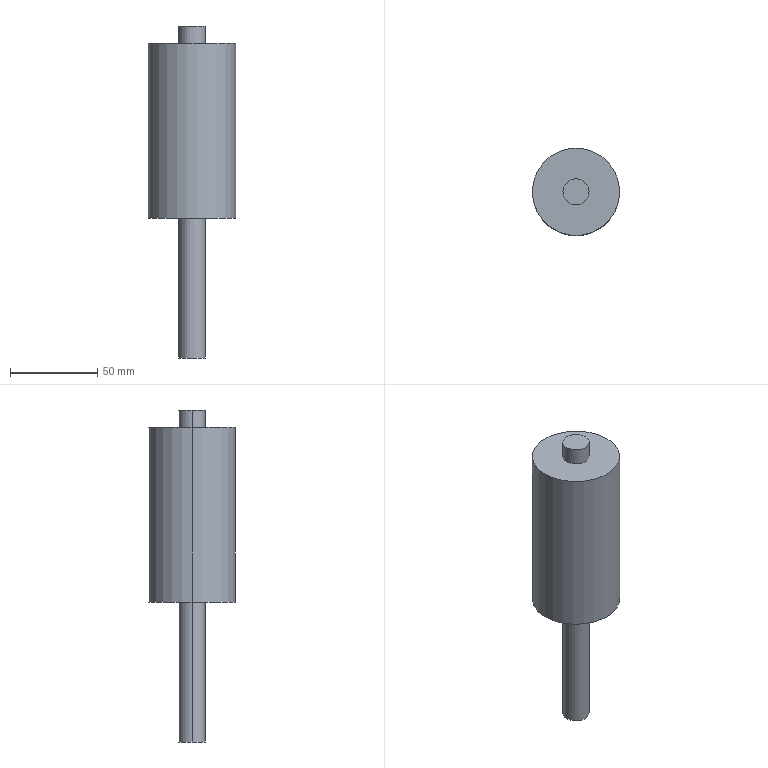Part | SolidWorks | features ICE 2, Extrusion 1 | 1 solid | 10 faces | box 50 x 50 x 190 mm | volume 212254 mm3 | cylinder 6 | plane 4 | commonest cylinder face diameters 15 x4 50 x2
STEP:
#1=CARTESIAN_POINT('',(-7.5,0.,-80.));
#2=VERTEX_POINT('',#1);
#3=CARTESIAN_POINT('',(7.5,0.,-80.));
#4=VERTEX_POINT('',#3);
#5=CARTESIAN_POINT('',(0.,0.,-80.));
#6=DIRECTION('',(0.,0.,-1.));
#7=DIRECTION('',(-1.,0.,0.));
#8=AXIS2_PLACEMENT_3D('',#5,#6,#7);
#9=CIRCLE('',#8,7.5);
#10=EDGE_CURVE('',#2,#4,#9,.T.);
#11=ORIENTED_EDGE('',*,*,#10,.F.);
#12=CARTESIAN_POINT('',(-7.5,0.,0.));
#13=VERTEX_POINT('',#12);
#14=CARTESIAN_POINT('',(-7.5,0.,-80.));
#15=DIRECTION('',(0.,0.,1.));
#16=VECTOR('',#15,1000.);
#17=LINE('',#14,#16);
#18=EDGE_CURVE('',#2,#13,#17,.T.);
#19=ORIENTED_EDGE('',*,*,#18,.T.);
#20=CARTESIAN_POINT('',(7.5,0.,0.));
#21=VERTEX_POINT('',#20);
#22=CARTESIAN_POINT('',(0.,0.,0.));
#23=DIRECTION('',(0.,0.,-1.));
#24=DIRECTION('',(-1.,0.,0.));
#25=AXIS2_PLACEMENT_3D('',#22,#23,#24);
#26=CIRCLE('',#25,7.5);
#27=EDGE_CURVE('',#13,#21,#26,.T.);
#28=ORIENTED_EDGE('',*,*,#27,.T.);
#29=CARTESIAN_POINT('',(7.5,0.,-80.));
#30=DIRECTION('',(0.,0.,1.));
#31=VECTOR('',#30,1000.);
#32=LINE('',#29,#31);
#33=EDGE_CURVE('',#4,#21,#32,.T.);
#34=ORIENTED_EDGE('',*,*,#33,.F.);
#35=EDGE_LOOP('',(#11,#19,#28,#34));
#36=FACE_OUTER_BOUND('',#35,.T.);
#37=CARTESIAN_POINT('',(0.,0.,-80.));
#38=DIRECTION('',(0.,0.,1.));
#39=DIRECTION('',(1.,0.,0.));
#40=AXIS2_PLACEMENT_3D('',#37,#38,#39);
#41=CYLINDRICAL_SURFACE('',#40,7.5);
#42=ADVANCED_FACE('',(#36),#41,.T.);
#43=CARTESIAN_POINT('',(7.5,0.,110.));
#44=VERTEX_POINT('',#43);
#45=CARTESIAN_POINT('',(-7.5,0.,110.));
#46=VERTEX_POINT('',#45);
#47=CARTESIAN_POINT('',(0.,0.,110.));
#48=DIRECTION('',(0.,0.,1.));
#49=DIRECTION('',(1.,0.,0.));
#50=AXIS2_PLACEMENT_3D('',#47,#48,#49);
#51=CIRCLE('',#50,7.5);
#52=EDGE_CURVE('',#44,#46,#51,.T.);
#53=ORIENTED_EDGE('',*,*,#52,.F.);
#54=CARTESIAN_POINT('',(7.5,0.,100.));
#55=VERTEX_POINT('',#54);
#56=CARTESIAN_POINT('',(7.5,0.,110.));
#57=DIRECTION('',(0.,0.,-1.));
#58=VECTOR('',#57,1000.);
#59=LINE('',#56,#58);
#60=EDGE_CURVE('',#44,#55,#59,.T.);
#61=ORIENTED_EDGE('',*,*,#60,.T.);
#62=CARTESIAN_POINT('',(-7.5,0.,100.));
#63=VERTEX_POINT('',#62);
#64=CARTESIAN_POINT('',(0.,0.,100.));
#65=DIRECTION('',(0.,0.,1.));
#66=DIRECTION('',(1.,0.,0.));
#67=AXIS2_PLACEMENT_3D('',#64,#65,#66);
#68=CIRCLE('',#67,7.5);
#69=EDGE_CURVE('',#55,#63,#68,.T.);
#70=ORIENTED_EDGE('',*,*,#69,.T.);
#71=CARTESIAN_POINT('',(-7.5,0.,110.));
#72=DIRECTION('',(0.,0.,-1.));
#73=VECTOR('',#72,1000.);
#74=LINE('',#71,#73);
#75=EDGE_CURVE('',#46,#63,#74,.T.);
#76=ORIENTED_EDGE('',*,*,#75,.F.);
#77=EDGE_LOOP('',(#53,#61,#70,#76));
#78=FACE_OUTER_BOUND('',#77,.T.);
#79=CARTESIAN_POINT('',(0.,0.,110.));
#80=DIRECTION('',(0.,0.,-1.));
#81=DIRECTION('',(-1.,0.,0.));
#82=AXIS2_PLACEMENT_3D('',#79,#80,#81);
#83=CYLINDRICAL_SURFACE('',#82,7.5);
#84=ADVANCED_FACE('',(#78),#83,.T.);
#85=CARTESIAN_POINT('',(25.,0.,100.));
#86=VERTEX_POINT('',#85);
#87=CARTESIAN_POINT('',(-25.,0.,100.));
#88=VERTEX_POINT('',#87);
#89=CARTESIAN_POINT('',(0.,0.,100.));
#90=DIRECTION('',(0.,0.,1.));
#91=DIRECTION('',(1.,0.,0.));
#92=AXIS2_PLACEMENT_3D('',#89,#90,#91);
#93=CIRCLE('',#92,25.);
#94=EDGE_CURVE('',#86,#88,#93,.T.);
#95=ORIENTED_EDGE('',*,*,#94,.F.);
#96=CARTESIAN_POINT('',(25.,0.,0.));
#97=VERTEX_POINT('',#96);
#98=CARTESIAN_POINT('',(25.,0.,100.));
#99=DIRECTION('',(0.,0.,-1.));
#100=VECTOR('',#99,1000.);
#101=LINE('',#98,#100);
#102=EDGE_CURVE('',#86,#97,#101,.T.);
#103=ORIENTED_EDGE('',*,*,#102,.T.);
#104=CARTESIAN_POINT('',(-25.,0.,0.));
#105=VERTEX_POINT('',#104);
#106=CARTESIAN_POINT('',(0.,0.,0.));
#107=DIRECTION('',(0.,0.,1.));
#108=DIRECTION('',(1.,0.,0.));
#109=AXIS2_PLACEMENT_3D('',#106,#107,#108);
#110=CIRCLE('',#109,25.);
#111=EDGE_CURVE('',#97,#105,#110,.T.);
#112=ORIENTED_EDGE('',*,*,#111,.T.);
#113=CARTESIAN_POINT('',(-25.,0.,100.));
#114=DIRECTION('',(0.,0.,-1.));
#115=VECTOR('',#114,1000.);
#116=LINE('',#113,#115);
#117=EDGE_CURVE('',#88,#105,#116,.T.);
#118=ORIENTED_EDGE('',*,*,#117,.F.);
#119=EDGE_LOOP('',(#95,#103,#112,#118));
#120=FACE_OUTER_BOUND('',#119,.T.);
#121=CARTESIAN_POINT('',(0.,0.,100.));
#122=DIRECTION('',(0.,0.,-1.));
#123=DIRECTION('',(-1.,0.,0.));
#124=AXIS2_PLACEMENT_3D('',#121,#122,#123);
#125=CYLINDRICAL_SURFACE('',#124,25.);
#126=ADVANCED_FACE('',(#120),#125,.T.);
#127=ORIENTED_EDGE('',*,*,#102,.F.);
#128=CARTESIAN_POINT('',(0.,0.,100.));
#129=DIRECTION('',(0.,0.,1.));
#130=DIRECTION('',(1.,0.,0.));
#131=AXIS2_PLACEMENT_3D('',#128,#129,#130);
#132=CIRCLE('',#131,25.);
#133=EDGE_CURVE('',#88,#86,#132,.T.);
#134=ORIENTED_EDGE('',*,*,#133,.F.);
#135=ORIENTED_EDGE('',*,*,#117,.T.);
#136=CARTESIAN_POINT('',(0.,0.,0.));
#137=DIRECTION('',(0.,0.,1.));
#138=DIRECTION('',(1.,0.,0.));
#139=AXIS2_PLACEMENT_3D('',#136,#137,#138);
#140=CIRCLE('',#139,25.);
#141=EDGE_CURVE('',#105,#97,#140,.T.);
#142=ORIENTED_EDGE('',*,*,#141,.T.);
#143=EDGE_LOOP('',(#127,#134,#135,#142));
#144=FACE_OUTER_BOUND('',#143,.T.);
#145=CARTESIAN_POINT('',(0.,0.,100.));
#146=DIRECTION('',(0.,0.,-1.));
#147=DIRECTION('',(-1.,0.,0.));
#148=AXIS2_PLACEMENT_3D('',#145,#146,#147);
#149=CYLINDRICAL_SURFACE('',#148,25.);
#150=ADVANCED_FACE('',(#144),#149,.T.);
#151=CARTESIAN_POINT('',(0.,0.,100.));
#152=DIRECTION('',(0.,0.,1.));
#153=DIRECTION('',(1.,0.,0.));
#154=AXIS2_PLACEMENT_3D('',#151,#152,#153);
#155=CIRCLE('',#154,7.5);
#156=EDGE_CURVE('',#63,#55,#155,.T.);
#157=ORIENTED_EDGE('',*,*,#156,.F.);
#158=ORIENTED_EDGE('',*,*,#69,.F.);
#159=EDGE_LOOP('',(#157,#158));
#160=FACE_BOUND('',#159,.T.);
#161=ORIENTED_EDGE('',*,*,#133,.T.);
#162=ORIENTED_EDGE('',*,*,#94,.T.);
#163=EDGE_LOOP('',(#161,#162));
#164=FACE_OUTER_BOUND('',#163,.T.);
#165=CARTESIAN_POINT('',(0.,0.,100.));
#166=DIRECTION('',(0.,0.,1.));
#167=DIRECTION('',(1.,0.,0.));
#168=AXIS2_PLACEMENT_3D('',#165,#166,#167);
#169=PLANE('',#168);
#170=ADVANCED_FACE('',(#160,#164),#169,.T.);
#171=CARTESIAN_POINT('',(0.,0.,0.));
#172=DIRECTION('',(0.,0.,-1.));
#173=DIRECTION('',(-1.,0.,0.));
#174=AXIS2_PLACEMENT_3D('',#171,#172,#173);
#175=CIRCLE('',#174,7.5);
#176=EDGE_CURVE('',#21,#13,#175,.T.);
#177=ORIENTED_EDGE('',*,*,#176,.F.);
#178=ORIENTED_EDGE('',*,*,#27,.F.);
#179=EDGE_LOOP('',(#177,#178));
#180=FACE_BOUND('',#179,.T.);
#181=ORIENTED_EDGE('',*,*,#141,.F.);
#182=ORIENTED_EDGE('',*,*,#111,.F.);
#183=EDGE_LOOP('',(#181,#182));
#184=FACE_OUTER_BOUND('',#183,.T.);
#185=CARTESIAN_POINT('',(0.,0.,0.));
#186=DIRECTION('',(0.,0.,1.));
#187=DIRECTION('',(1.,0.,0.));
#188=AXIS2_PLACEMENT_3D('',#185,#186,#187);
#189=PLANE('',#188);
#190=ADVANCED_FACE('',(#180,#184),#189,.F.);
#191=ORIENTED_EDGE('',*,*,#60,.F.);
#192=CARTESIAN_POINT('',(0.,0.,110.));
#193=DIRECTION('',(0.,0.,1.));
#194=DIRECTION('',(1.,0.,0.));
#195=AXIS2_PLACEMENT_3D('',#192,#193,#194);
#196=CIRCLE('',#195,7.5);
#197=EDGE_CURVE('',#46,#44,#196,.T.);
#198=ORIENTED_EDGE('',*,*,#197,.F.);
#199=ORIENTED_EDGE('',*,*,#75,.T.);
#200=ORIENTED_EDGE('',*,*,#156,.T.);
#201=EDGE_LOOP('',(#191,#198,#199,#200));
#202=FACE_OUTER_BOUND('',#201,.T.);
#203=CARTESIAN_POINT('',(0.,0.,110.));
#204=DIRECTION('',(0.,0.,-1.));
#205=DIRECTION('',(-1.,0.,0.));
#206=AXIS2_PLACEMENT_3D('',#203,#204,#205);
#207=CYLINDRICAL_SURFACE('',#206,7.5);
#208=ADVANCED_FACE('',(#202),#207,.T.);
#209=ORIENTED_EDGE('',*,*,#197,.T.);
#210=ORIENTED_EDGE('',*,*,#52,.T.);
#211=EDGE_LOOP('',(#209,#210));
#212=FACE_OUTER_BOUND('',#211,.T.);
#213=CARTESIAN_POINT('',(0.,0.,110.));
#214=DIRECTION('',(0.,0.,1.));
#215=DIRECTION('',(1.,0.,0.));
#216=AXIS2_PLACEMENT_3D('',#213,#214,#215);
#217=PLANE('',#216);
#218=ADVANCED_FACE('',(#212),#217,.T.);
#219=ORIENTED_EDGE('',*,*,#18,.F.);
#220=CARTESIAN_POINT('',(0.,0.,-80.));
#221=DIRECTION('',(0.,0.,-1.));
#222=DIRECTION('',(-1.,0.,0.));
#223=AXIS2_PLACEMENT_3D('',#220,#221,#222);
#224=CIRCLE('',#223,7.5);
#225=EDGE_CURVE('',#4,#2,#224,.T.);
#226=ORIENTED_EDGE('',*,*,#225,.F.);
#227=ORIENTED_EDGE('',*,*,#33,.T.);
#228=ORIENTED_EDGE('',*,*,#176,.T.);
#229=EDGE_LOOP('',(#219,#226,#227,#228));
#230=FACE_OUTER_BOUND('',#229,.T.);
#231=CARTESIAN_POINT('',(0.,0.,-80.));
#232=DIRECTION('',(0.,0.,1.));
#233=DIRECTION('',(1.,0.,0.));
#234=AXIS2_PLACEMENT_3D('',#231,#232,#233);
#235=CYLINDRICAL_SURFACE('',#234,7.5);
#236=ADVANCED_FACE('',(#230),#235,.T.);
#237=ORIENTED_EDGE('',*,*,#225,.T.);
#238=ORIENTED_EDGE('',*,*,#10,.T.);
#239=EDGE_LOOP('',(#237,#238));
#240=FACE_OUTER_BOUND('',#239,.T.);
#241=CARTESIAN_POINT('',(0.,0.,-80.));
#242=DIRECTION('',(0.,0.,-1.));
#243=DIRECTION('',(-1.,0.,0.));
#244=AXIS2_PLACEMENT_3D('',#241,#242,#243);
#245=PLANE('',#244);
#246=ADVANCED_FACE('',(#240),#245,.T.);
#247=CLOSED_SHELL('',(#42,#84,#126,#150,#170,#190,#208,#218,#236,#246));
#248=MANIFOLD_SOLID_BREP('',#247);
#249=CARTESIAN_POINT('',(0.,0.,0.));
#250=DIRECTION('',(0.,0.,1.));
#251=DIRECTION('',(1.,0.,0.));
#252=AXIS2_PLACEMENT_3D('',#249,#250,#251);
#253=(LENGTH_UNIT()NAMED_UNIT(*)SI_UNIT(.MILLI.,.METRE.));
#254=UNCERTAINTY_MEASURE_WITH_UNIT(LENGTH_MEASURE(0.00001),#253,'','');
#255=(NAMED_UNIT(*)PLANE_ANGLE_UNIT()SI_UNIT($,.RADIAN.));
#256=(NAMED_UNIT(*)SI_UNIT($,.STERADIAN.)SOLID_ANGLE_UNIT());
#257=(GEOMETRIC_REPRESENTATION_CONTEXT(3)GLOBAL_UNCERTAINTY_ASSIGNED_CONTEXT((#254))GLOBAL_UNIT_ASSIGNED_CONTEXT((#253,#255,#256))REPRESENTATION_CONTEXT('',''));
#258=ADVANCED_BREP_SHAPE_REPRESENTATION('',(#248,#252),#257);